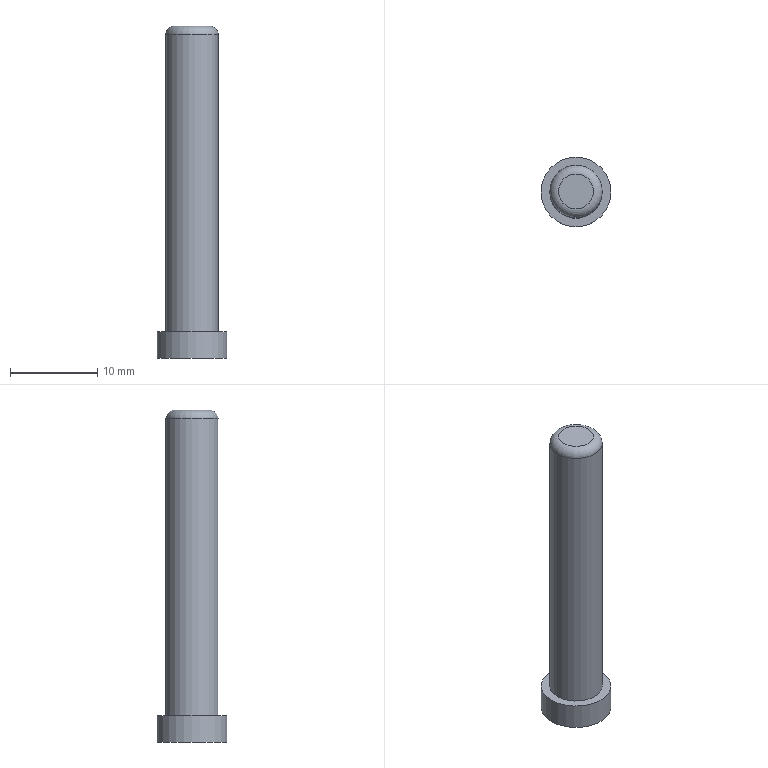Part | STEP file | 6-35_id1846_x_t | 1 solid | 6 faces | box 8 x 8 x 38 mm | volume 1137 mm3 | plane 3 | cylinder 2 | torus 1 | commonest cylinder face diameters 6.001 x1 8 x1
STEP:
#1=CARTESIAN_POINT('',(345.,-22.5,2.));
#2=VERTEX_POINT('',#1);
#3=CARTESIAN_POINT('',(342.,-22.5,2.));
#4=DIRECTION('',(0.,0.,-1.));
#5=DIRECTION('',(1.,0.,0.));
#6=AXIS2_PLACEMENT_3D('',#3,#4,#5);
#7=CIRCLE('',#6,3.001);
#8=EDGE_CURVE('',#2,#2,#7,.T.);
#9=ORIENTED_EDGE('',*,*,#8,.T.);
#10=EDGE_LOOP('',(#9));
#11=FACE_BOUND('',#10,.T.);
#12=CARTESIAN_POINT('',(345.,-22.5,-32.));
#13=VERTEX_POINT('',#12);
#14=CARTESIAN_POINT('',(342.,-22.5,-32.));
#15=DIRECTION('',(0.,0.,-1.));
#16=DIRECTION('',(1.,0.,0.));
#17=AXIS2_PLACEMENT_3D('',#14,#15,#16);
#18=CIRCLE('',#17,3.001);
#19=EDGE_CURVE('',#13,#13,#18,.T.);
#20=ORIENTED_EDGE('',*,*,#19,.F.);
#21=EDGE_LOOP('',(#20));
#22=FACE_BOUND('',#21,.T.);
#23=CARTESIAN_POINT('',(342.,-22.5,-2.));
#24=DIRECTION('',(0.,0.,-1.));
#25=DIRECTION('',(-1.,0.,0.));
#26=AXIS2_PLACEMENT_3D('',#23,#24,#25);
#27=CYLINDRICAL_SURFACE('',#26,3.001);
#28=ADVANCED_FACE('',(#11,#22),#27,.T.);
#29=CARTESIAN_POINT('',(344.,-22.5,3.));
#30=VERTEX_POINT('',#29);
#31=CARTESIAN_POINT('',(342.,-22.5,3.));
#32=DIRECTION('',(0.,0.,1.));
#33=DIRECTION('',(1.,0.,0.));
#34=AXIS2_PLACEMENT_3D('',#31,#32,#33);
#35=CIRCLE('',#34,2.001);
#36=EDGE_CURVE('',#30,#30,#35,.T.);
#37=ORIENTED_EDGE('',*,*,#36,.T.);
#38=EDGE_LOOP('',(#37));
#39=FACE_OUTER_BOUND('',#38,.T.);
#40=CARTESIAN_POINT('',(342.,-22.5,3.));
#41=DIRECTION('',(0.,0.,1.));
#42=DIRECTION('',(1.,0.,0.));
#43=AXIS2_PLACEMENT_3D('',#40,#41,#42);
#44=PLANE('',#43);
#45=ADVANCED_FACE('',(#39),#44,.T.);
#46=CARTESIAN_POINT('',(338.,-22.5,-35.));
#47=VERTEX_POINT('',#46);
#48=CARTESIAN_POINT('',(342.,-22.5,-35.));
#49=DIRECTION('',(0.,0.,1.));
#50=DIRECTION('',(-1.,0.,0.));
#51=AXIS2_PLACEMENT_3D('',#48,#49,#50);
#52=CIRCLE('',#51,4.);
#53=EDGE_CURVE('',#47,#47,#52,.T.);
#54=ORIENTED_EDGE('',*,*,#53,.F.);
#55=EDGE_LOOP('',(#54));
#56=FACE_OUTER_BOUND('',#55,.T.);
#57=CARTESIAN_POINT('',(342.,-22.5,-35.));
#58=DIRECTION('',(0.,0.,-1.));
#59=DIRECTION('',(-1.,0.,0.));
#60=AXIS2_PLACEMENT_3D('',#57,#58,#59);
#61=PLANE('',#60);
#62=ADVANCED_FACE('',(#56),#61,.T.);
#63=ORIENTED_EDGE('',*,*,#19,.T.);
#64=EDGE_LOOP('',(#63));
#65=FACE_BOUND('',#64,.T.);
#66=CARTESIAN_POINT('',(338.,-22.5,-32.));
#67=VERTEX_POINT('',#66);
#68=CARTESIAN_POINT('',(342.,-22.5,-32.));
#69=DIRECTION('',(0.,0.,-1.));
#70=DIRECTION('',(-1.,0.,0.));
#71=AXIS2_PLACEMENT_3D('',#68,#69,#70);
#72=CIRCLE('',#71,4.);
#73=EDGE_CURVE('',#67,#67,#72,.T.);
#74=ORIENTED_EDGE('',*,*,#73,.F.);
#75=EDGE_LOOP('',(#74));
#76=FACE_BOUND('',#75,.T.);
#77=CARTESIAN_POINT('',(342.,-22.5,-32.));
#78=DIRECTION('',(0.,0.,1.));
#79=DIRECTION('',(1.,0.,0.));
#80=AXIS2_PLACEMENT_3D('',#77,#78,#79);
#81=PLANE('',#80);
#82=ADVANCED_FACE('',(#65,#76),#81,.T.);
#83=ORIENTED_EDGE('',*,*,#53,.T.);
#84=EDGE_LOOP('',(#83));
#85=FACE_BOUND('',#84,.T.);
#86=ORIENTED_EDGE('',*,*,#73,.T.);
#87=EDGE_LOOP('',(#86));
#88=FACE_BOUND('',#87,.T.);
#89=CARTESIAN_POINT('',(342.,-22.5,-32.));
#90=DIRECTION('',(0.,0.,-1.));
#91=DIRECTION('',(-1.,0.,0.));
#92=AXIS2_PLACEMENT_3D('',#89,#90,#91);
#93=CYLINDRICAL_SURFACE('',#92,4.);
#94=ADVANCED_FACE('',(#85,#88),#93,.T.);
#95=ORIENTED_EDGE('',*,*,#36,.F.);
#96=EDGE_LOOP('',(#95));
#97=FACE_BOUND('',#96,.T.);
#98=ORIENTED_EDGE('',*,*,#8,.F.);
#99=EDGE_LOOP('',(#98));
#100=FACE_BOUND('',#99,.T.);
#101=CARTESIAN_POINT('',(342.,-22.5,2.));
#102=DIRECTION('',(0.,0.,1.));
#103=DIRECTION('',(1.,0.,0.));
#104=AXIS2_PLACEMENT_3D('',#101,#102,#103);
#105=TOROIDAL_SURFACE('',#104,2.001,1.);
#106=ADVANCED_FACE('',(#97,#100),#105,.T.);
#107=CLOSED_SHELL('',(#28,#45,#62,#82,#94,#106));
#108=MANIFOLD_SOLID_BREP('',#107);
#109=(LENGTH_UNIT()NAMED_UNIT(*)SI_UNIT(.MILLI.,.METRE.));
#110=UNCERTAINTY_MEASURE_WITH_UNIT(LENGTH_MEASURE(0.00002),#109,'','');
#111=(NAMED_UNIT(*)PLANE_ANGLE_UNIT()SI_UNIT($,.RADIAN.));
#112=PLANE_ANGLE_MEASURE_WITH_UNIT(PLANE_ANGLE_MEASURE(0.01745),#111);
#113=DIMENSIONAL_EXPONENTS(0.,0.,0.,0.,0.,0.,0.);
#114=(CONVERSION_BASED_UNIT('DEGREE',#112)NAMED_UNIT(#113)PLANE_ANGLE_UNIT());
#115=(NAMED_UNIT(*)SI_UNIT($,.STERADIAN.)SOLID_ANGLE_UNIT());
#116=(GEOMETRIC_REPRESENTATION_CONTEXT(3)GLOBAL_UNCERTAINTY_ASSIGNED_CONTEXT((#110))GLOBAL_UNIT_ASSIGNED_CONTEXT((#109,#114,#115))REPRESENTATION_CONTEXT('',''));
#117=ADVANCED_BREP_SHAPE_REPRESENTATION('',(#108),#116);